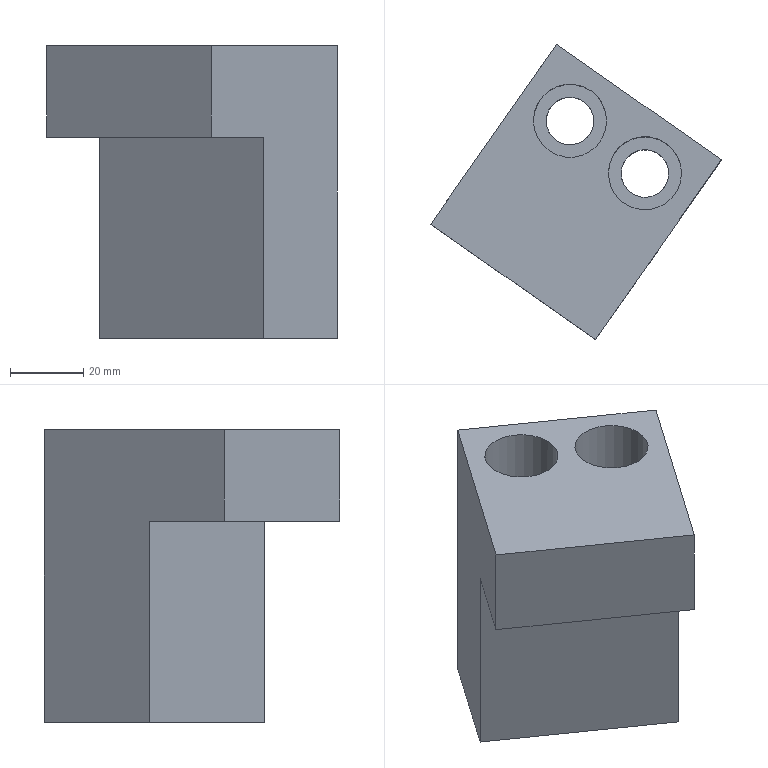Part | NX | features solid 2 | 1 solid | 14 faces | box 79.468 x 80.696 x 80 mm | volume 148999 mm3 | plane 9 | cylinder 4 | spline 1 | commonest cylinder face diameters 13 x2 20 x2
STEP:
#1=CARTESIAN_POINT('',(301.621,356.463,-125.));
#2=VERTEX_POINT('',#1);
#3=CARTESIAN_POINT('',(256.568,388.01,-125.));
#4=VERTEX_POINT('',#3);
#5=CARTESIAN_POINT('',(791.825,13.218,-125.));
#6=DIRECTION('',(-0.8192,0.5736,0.));
#7=VECTOR('',#6,1000.);
#8=LINE('',#5,#7);
#9=EDGE_CURVE('',#2,#4,#8,.T.);
#10=ORIENTED_EDGE('',*,*,#9,.F.);
#11=CARTESIAN_POINT('',(287.282,335.984,-125.));
#12=VERTEX_POINT('',#11);
#13=CARTESIAN_POINT('',(281.546,327.793,-125.));
#14=DIRECTION('',(-0.5736,-0.8192,0.));
#15=VECTOR('',#14,1000.);
#16=LINE('',#13,#15);
#17=EDGE_CURVE('',#12,#2,#16,.F.);
#18=ORIENTED_EDGE('',*,*,#17,.F.);
#19=CARTESIAN_POINT('',(242.228,367.531,-125.));
#20=VERTEX_POINT('',#19);
#21=CARTESIAN_POINT('',(283.186,338.852,-125.));
#22=DIRECTION('',(0.8192,-0.5736,0.));
#23=VECTOR('',#22,1000.);
#24=LINE('',#21,#23);
#25=EDGE_CURVE('',#12,#20,#24,.F.);
#26=ORIENTED_EDGE('',*,*,#25,.T.);
#27=CARTESIAN_POINT('',(-24.693,-13.672,-125.));
#28=DIRECTION('',(-0.5736,-0.8192,0.));
#29=VECTOR('',#28,1000.);
#30=LINE('',#27,#29);
#31=EDGE_CURVE('',#20,#4,#30,.F.);
#32=ORIENTED_EDGE('',*,*,#31,.T.);
#33=EDGE_LOOP('',(#10,#18,#26,#32));
#34=FACE_BOUND('',#33,.T.);
#35=CARTESIAN_POINT('',(510.565,-388.463,-125.));
#36=DIRECTION('',(0.,0.,-1.));
#37=DIRECTION('',(-0.342,0.9397,0.));
#38=AXIS2_PLACEMENT_3D('',#35,#36,#37);
#39=PLANE('',#38);
#40=ADVANCED_FACE('',(#34),#39,.T.);
#41=ORIENTED_EDGE('',*,*,#25,.F.);
#42=CARTESIAN_POINT('',(287.282,335.984,-100.));
#43=VERTEX_POINT('',#42);
#44=CARTESIAN_POINT('',(287.282,335.984,-100.));
#45=DIRECTION('',(0.,0.,-1.));
#46=VECTOR('',#45,1000.);
#47=LINE('',#44,#46);
#48=EDGE_CURVE('',#43,#12,#47,.T.);
#49=ORIENTED_EDGE('',*,*,#48,.F.);
#50=CARTESIAN_POINT('',(242.228,367.531,-100.));
#51=VERTEX_POINT('',#50);
#52=CARTESIAN_POINT('',(283.186,338.852,-100.));
#53=DIRECTION('',(0.8192,-0.5736,0.));
#54=VECTOR('',#53,1000.);
#55=LINE('',#52,#54);
#56=EDGE_CURVE('',#43,#51,#55,.F.);
#57=ORIENTED_EDGE('',*,*,#56,.T.);
#58=CARTESIAN_POINT('',(242.228,367.531,-100.));
#59=DIRECTION('',(0.,0.,-1.));
#60=VECTOR('',#59,1000.);
#61=LINE('',#58,#60);
#62=EDGE_CURVE('',#51,#20,#61,.T.);
#63=ORIENTED_EDGE('',*,*,#62,.T.);
#64=EDGE_LOOP('',(#41,#49,#57,#63));
#65=FACE_BOUND('',#64,.T.);
#66=CARTESIAN_POINT('',(283.186,338.852,-100.));
#67=DIRECTION('',(0.5736,0.8192,0.));
#68=DIRECTION('',(0.8192,-0.5736,0.));
#69=AXIS2_PLACEMENT_3D('',#66,#67,#68);
#70=PLANE('',#69);
#71=ADVANCED_FACE('',(#65),#70,.F.);
#72=ORIENTED_EDGE('',*,*,#31,.F.);
#73=ORIENTED_EDGE('',*,*,#62,.F.);
#74=CARTESIAN_POINT('',(276.643,416.68,-100.));
#75=VERTEX_POINT('',#74);
#76=CARTESIAN_POINT('',(-24.693,-13.672,-100.));
#77=DIRECTION('',(-0.5736,-0.8192,0.));
#78=VECTOR('',#77,1000.);
#79=LINE('',#76,#78);
#80=EDGE_CURVE('',#51,#75,#79,.F.);
#81=ORIENTED_EDGE('',*,*,#80,.T.);
#82=CARTESIAN_POINT('',(276.643,416.68,-180.));
#83=VERTEX_POINT('',#82);
#84=CARTESIAN_POINT('',(276.643,416.68,-100.));
#85=DIRECTION('',(0.,0.,-1.));
#86=VECTOR('',#85,1000.);
#87=LINE('',#84,#86);
#88=EDGE_CURVE('',#75,#83,#87,.T.);
#89=ORIENTED_EDGE('',*,*,#88,.T.);
#90=CARTESIAN_POINT('',(256.568,388.01,-180.));
#91=VERTEX_POINT('',#90);
#92=CARTESIAN_POINT('',(256.568,388.01,-180.));
#93=CARTESIAN_POINT('',(263.259,397.566,-180.));
#94=CARTESIAN_POINT('',(269.951,407.123,-180.));
#95=CARTESIAN_POINT('',(276.643,416.68,-180.));
#96=B_SPLINE_CURVE_WITH_KNOTS('',3,(#92,#93,#94,#95),.UNSPECIFIED.,.F.,.F.,(4,4),(0.,0.035),.UNSPECIFIED.);
#97=EDGE_CURVE('',#91,#83,#96,.T.);
#98=ORIENTED_EDGE('',*,*,#97,.F.);
#99=CARTESIAN_POINT('',(256.568,388.01,-175.));
#100=DIRECTION('',(0.,0.,-1.));
#101=VECTOR('',#100,1000.);
#102=LINE('',#99,#101);
#103=EDGE_CURVE('',#91,#4,#102,.F.);
#104=ORIENTED_EDGE('',*,*,#103,.T.);
#105=EDGE_LOOP('',(#72,#73,#81,#89,#98,#104));
#106=FACE_BOUND('',#105,.T.);
#107=CARTESIAN_POINT('',(-24.693,-13.672,-100.));
#108=DIRECTION('',(0.8192,-0.5736,0.));
#109=DIRECTION('',(-0.5736,-0.8192,0.));
#110=AXIS2_PLACEMENT_3D('',#107,#108,#109);
#111=PLANE('',#110);
#112=ADVANCED_FACE('',(#106),#111,.F.);
#113=CARTESIAN_POINT('',(321.696,385.133,-100.));
#114=VERTEX_POINT('',#113);
#115=CARTESIAN_POINT('',(321.696,385.133,-180.));
#116=VERTEX_POINT('',#115);
#117=CARTESIAN_POINT('',(321.696,385.133,-100.));
#118=DIRECTION('',(0.,0.,-1.));
#119=VECTOR('',#118,1000.);
#120=LINE('',#117,#119);
#121=EDGE_CURVE('',#114,#116,#120,.T.);
#122=ORIENTED_EDGE('',*,*,#121,.T.);
#123=CARTESIAN_POINT('',(321.696,385.133,-180.));
#124=CARTESIAN_POINT('',(306.678,395.649,-180.));
#125=CARTESIAN_POINT('',(291.661,406.164,-180.));
#126=CARTESIAN_POINT('',(276.643,416.68,-180.));
#127=B_SPLINE_CURVE_WITH_KNOTS('',3,(#123,#124,#125,#126),.UNSPECIFIED.,.F.,.F.,(4,4),(0.,0.055),.UNSPECIFIED.);
#128=EDGE_CURVE('',#116,#83,#127,.T.);
#129=ORIENTED_EDGE('',*,*,#128,.T.);
#130=ORIENTED_EDGE('',*,*,#88,.F.);
#131=CARTESIAN_POINT('',(313.505,390.869,-100.));
#132=DIRECTION('',(0.8192,-0.5736,0.));
#133=VECTOR('',#132,1000.);
#134=LINE('',#131,#133);
#135=EDGE_CURVE('',#114,#75,#134,.F.);
#136=ORIENTED_EDGE('',*,*,#135,.F.);
#137=EDGE_LOOP('',(#122,#129,#130,#136));
#138=FACE_BOUND('',#137,.T.);
#139=CARTESIAN_POINT('',(313.505,390.869,-15.));
#140=DIRECTION('',(0.5736,0.8192,0.));
#141=DIRECTION('',(0.8192,-0.5736,0.));
#142=AXIS2_PLACEMENT_3D('',#139,#140,#141);
#143=PLANE('',#142);
#144=ADVANCED_FACE('',(#138),#143,.T.);
#145=ORIENTED_EDGE('',*,*,#17,.T.);
#146=CARTESIAN_POINT('',(301.621,356.463,-180.));
#147=VERTEX_POINT('',#146);
#148=CARTESIAN_POINT('',(301.621,356.463,-175.));
#149=DIRECTION('',(0.,0.,-1.));
#150=VECTOR('',#149,1000.);
#151=LINE('',#148,#150);
#152=EDGE_CURVE('',#147,#2,#151,.F.);
#153=ORIENTED_EDGE('',*,*,#152,.F.);
#154=CARTESIAN_POINT('',(301.621,356.463,-180.));
#155=CARTESIAN_POINT('',(308.313,366.02,-180.));
#156=CARTESIAN_POINT('',(315.005,375.576,-180.));
#157=CARTESIAN_POINT('',(321.696,385.133,-180.));
#158=B_SPLINE_CURVE_WITH_KNOTS('',3,(#154,#155,#156,#157),.UNSPECIFIED.,.F.,.F.,(4,4),(0.,0.035),.UNSPECIFIED.);
#159=EDGE_CURVE('',#147,#116,#158,.T.);
#160=ORIENTED_EDGE('',*,*,#159,.T.);
#161=ORIENTED_EDGE('',*,*,#121,.F.);
#162=CARTESIAN_POINT('',(281.546,327.793,-100.));
#163=DIRECTION('',(-0.5736,-0.8192,0.));
#164=VECTOR('',#163,1000.);
#165=LINE('',#162,#164);
#166=EDGE_CURVE('',#43,#114,#165,.F.);
#167=ORIENTED_EDGE('',*,*,#166,.F.);
#168=ORIENTED_EDGE('',*,*,#48,.T.);
#169=EDGE_LOOP('',(#145,#153,#160,#161,#167,#168));
#170=FACE_BOUND('',#169,.T.);
#171=CARTESIAN_POINT('',(281.546,327.793,-100.));
#172=DIRECTION('',(0.8192,-0.5736,0.));
#173=DIRECTION('',(-0.5736,-0.8192,0.));
#174=AXIS2_PLACEMENT_3D('',#171,#172,#173);
#175=PLANE('',#174);
#176=ADVANCED_FACE('',(#170),#175,.T.);
#177=CARTESIAN_POINT('',(297.385,390.846,-100.));
#178=VERTEX_POINT('',#177);
#179=CARTESIAN_POINT('',(300.805,381.45,-100.));
#180=DIRECTION('',(0.,0.,1.));
#181=DIRECTION('',(-0.342,0.9397,0.));
#182=AXIS2_PLACEMENT_3D('',#179,#180,#181);
#183=CIRCLE('',#182,10.);
#184=EDGE_CURVE('',#178,#178,#183,.F.);
#185=ORIENTED_EDGE('',*,*,#184,.T.);
#186=EDGE_LOOP('',(#185));
#187=FACE_BOUND('',#186,.T.);
#188=CARTESIAN_POINT('',(276.906,405.186,-100.));
#189=VERTEX_POINT('',#188);
#190=CARTESIAN_POINT('',(280.326,395.789,-100.));
#191=DIRECTION('',(0.,0.,1.));
#192=DIRECTION('',(-0.342,0.9397,0.));
#193=AXIS2_PLACEMENT_3D('',#190,#191,#192);
#194=CIRCLE('',#193,10.);
#195=EDGE_CURVE('',#189,#189,#194,.F.);
#196=ORIENTED_EDGE('',*,*,#195,.T.);
#197=EDGE_LOOP('',(#196));
#198=FACE_BOUND('',#197,.T.);
#199=ORIENTED_EDGE('',*,*,#56,.F.);
#200=ORIENTED_EDGE('',*,*,#166,.T.);
#201=ORIENTED_EDGE('',*,*,#135,.T.);
#202=ORIENTED_EDGE('',*,*,#80,.F.);
#203=EDGE_LOOP('',(#199,#200,#201,#202));
#204=FACE_BOUND('',#203,.T.);
#205=CARTESIAN_POINT('',(510.565,-388.463,-100.));
#206=DIRECTION('',(0.,0.,-1.));
#207=DIRECTION('',(-0.342,0.9397,0.));
#208=AXIS2_PLACEMENT_3D('',#205,#206,#207);
#209=PLANE('',#208);
#210=ADVANCED_FACE('',(#187,#198,#204),#209,.F.);
#211=CARTESIAN_POINT('',(273.826,395.789,-150.));
#212=VERTEX_POINT('',#211);
#213=CARTESIAN_POINT('',(280.326,395.789,-150.));
#214=DIRECTION('',(0.,0.,-1.));
#215=DIRECTION('',(-1.,0.,0.));
#216=AXIS2_PLACEMENT_3D('',#213,#214,#215);
#217=CIRCLE('',#216,6.5);
#218=EDGE_CURVE('',#212,#212,#217,.T.);
#219=ORIENTED_EDGE('',*,*,#218,.F.);
#220=EDGE_LOOP('',(#219));
#221=FACE_BOUND('',#220,.T.);
#222=CARTESIAN_POINT('',(282.55,389.681,-180.));
#223=VERTEX_POINT('',#222);
#224=CARTESIAN_POINT('',(286.859,392.75,-180.));
#225=CARTESIAN_POINT('',(282.789,389.018,-180.));
#226=CARTESIAN_POINT('',(277.281,389.263,-180.));
#227=CARTESIAN_POINT('',(273.56,393.321,-180.));
#228=CARTESIAN_POINT('',(273.795,398.83,-180.));
#229=CARTESIAN_POINT('',(277.862,402.557,-180.));
#230=CARTESIAN_POINT('',(283.363,402.32,-180.));
#231=CARTESIAN_POINT('',(287.093,398.26,-180.));
#232=CARTESIAN_POINT('',(286.859,392.75,-180.));
#233=CARTESIAN_POINT('',(282.789,389.018,-180.));
#234=CARTESIAN_POINT('',(277.281,389.263,-180.));
#235=B_SPLINE_CURVE_WITH_KNOTS('',3,(#224,#225,#226,#227,#228,#229,#230,#231,#232,#233,#234),.UNSPECIFIED.,.T.,.F.,(1,1,1,1,1,1,1,1,1,1,1,1,1,1,1),(-0.01524,-0.01016,-0.00508,0.,0.00508,0.01016,0.01524,0.02032,0.0254,0.03048,0.03556,0.04064,0.04572,0.0508,0.05588),.UNSPECIFIED.);
#236=EDGE_CURVE('',#223,#223,#235,.T.);
#237=ORIENTED_EDGE('',*,*,#236,.T.);
#238=EDGE_LOOP('',(#237));
#239=FACE_BOUND('',#238,.T.);
#240=CARTESIAN_POINT('',(280.326,395.789,-145.));
#241=DIRECTION('',(0.,0.,1.));
#242=DIRECTION('',(0.342,-0.9397,0.));
#243=AXIS2_PLACEMENT_3D('',#240,#241,#242);
#244=CYLINDRICAL_SURFACE('',#243,6.5);
#245=ADVANCED_FACE('',(#221,#239),#244,.F.);
#246=ORIENTED_EDGE('',*,*,#218,.T.);
#247=EDGE_LOOP('',(#246));
#248=FACE_BOUND('',#247,.T.);
#249=CARTESIAN_POINT('',(270.326,395.789,-150.));
#250=VERTEX_POINT('',#249);
#251=CARTESIAN_POINT('',(280.326,395.789,-150.));
#252=DIRECTION('',(0.,0.,-1.));
#253=DIRECTION('',(-1.,0.,0.));
#254=AXIS2_PLACEMENT_3D('',#251,#252,#253);
#255=CIRCLE('',#254,10.);
#256=EDGE_CURVE('',#250,#250,#255,.T.);
#257=ORIENTED_EDGE('',*,*,#256,.F.);
#258=EDGE_LOOP('',(#257));
#259=FACE_BOUND('',#258,.T.);
#260=CARTESIAN_POINT('',(280.326,395.789,-150.));
#261=DIRECTION('',(0.,0.,-1.));
#262=DIRECTION('',(-0.342,0.9397,0.));
#263=AXIS2_PLACEMENT_3D('',#260,#261,#262);
#264=PLANE('',#263);
#265=ADVANCED_FACE('',(#248,#259),#264,.F.);
#266=ORIENTED_EDGE('',*,*,#195,.F.);
#267=EDGE_LOOP('',(#266));
#268=FACE_BOUND('',#267,.T.);
#269=ORIENTED_EDGE('',*,*,#256,.T.);
#270=EDGE_LOOP('',(#269));
#271=FACE_BOUND('',#270,.T.);
#272=CARTESIAN_POINT('',(280.326,395.789,-105.));
#273=DIRECTION('',(0.,0.,1.));
#274=DIRECTION('',(0.342,-0.9397,0.));
#275=AXIS2_PLACEMENT_3D('',#272,#273,#274);
#276=CYLINDRICAL_SURFACE('',#275,10.);
#277=ADVANCED_FACE('',(#268,#271),#276,.F.);
#278=CARTESIAN_POINT('',(294.305,381.45,-150.));
#279=VERTEX_POINT('',#278);
#280=CARTESIAN_POINT('',(300.805,381.45,-150.));
#281=DIRECTION('',(0.,0.,-1.));
#282=DIRECTION('',(-1.,0.,0.));
#283=AXIS2_PLACEMENT_3D('',#280,#281,#282);
#284=CIRCLE('',#283,6.5);
#285=EDGE_CURVE('',#279,#279,#284,.T.);
#286=ORIENTED_EDGE('',*,*,#285,.F.);
#287=EDGE_LOOP('',(#286));
#288=FACE_BOUND('',#287,.T.);
#289=CARTESIAN_POINT('',(303.028,375.342,-180.));
#290=VERTEX_POINT('',#289);
#291=CARTESIAN_POINT('',(307.338,378.411,-180.));
#292=CARTESIAN_POINT('',(303.268,374.679,-180.));
#293=CARTESIAN_POINT('',(297.76,374.923,-180.));
#294=CARTESIAN_POINT('',(294.039,378.981,-180.));
#295=CARTESIAN_POINT('',(294.274,384.491,-180.));
#296=CARTESIAN_POINT('',(298.341,388.217,-180.));
#297=CARTESIAN_POINT('',(303.842,387.98,-180.));
#298=CARTESIAN_POINT('',(307.572,383.921,-180.));
#299=CARTESIAN_POINT('',(307.338,378.411,-180.));
#300=CARTESIAN_POINT('',(303.268,374.679,-180.));
#301=CARTESIAN_POINT('',(297.76,374.923,-180.));
#302=B_SPLINE_CURVE_WITH_KNOTS('',3,(#291,#292,#293,#294,#295,#296,#297,#298,#299,#300,#301),.UNSPECIFIED.,.T.,.F.,(1,1,1,1,1,1,1,1,1,1,1,1,1,1,1),(-0.01524,-0.01016,-0.00508,0.,0.00508,0.01016,0.01524,0.02032,0.0254,0.03048,0.03556,0.04064,0.04572,0.0508,0.05588),.UNSPECIFIED.);
#303=EDGE_CURVE('',#290,#290,#302,.T.);
#304=ORIENTED_EDGE('',*,*,#303,.T.);
#305=EDGE_LOOP('',(#304));
#306=FACE_BOUND('',#305,.T.);
#307=CARTESIAN_POINT('',(300.805,381.45,-145.));
#308=DIRECTION('',(0.,0.,1.));
#309=DIRECTION('',(0.342,-0.9397,0.));
#310=AXIS2_PLACEMENT_3D('',#307,#308,#309);
#311=CYLINDRICAL_SURFACE('',#310,6.5);
#312=ADVANCED_FACE('',(#288,#306),#311,.F.);
#313=ORIENTED_EDGE('',*,*,#285,.T.);
#314=EDGE_LOOP('',(#313));
#315=FACE_BOUND('',#314,.T.);
#316=CARTESIAN_POINT('',(290.805,381.45,-150.));
#317=VERTEX_POINT('',#316);
#318=CARTESIAN_POINT('',(300.805,381.45,-150.));
#319=DIRECTION('',(0.,0.,-1.));
#320=DIRECTION('',(-1.,0.,0.));
#321=AXIS2_PLACEMENT_3D('',#318,#319,#320);
#322=CIRCLE('',#321,10.);
#323=EDGE_CURVE('',#317,#317,#322,.T.);
#324=ORIENTED_EDGE('',*,*,#323,.F.);
#325=EDGE_LOOP('',(#324));
#326=FACE_BOUND('',#325,.T.);
#327=CARTESIAN_POINT('',(300.805,381.45,-150.));
#328=DIRECTION('',(0.,0.,-1.));
#329=DIRECTION('',(-0.342,0.9397,0.));
#330=AXIS2_PLACEMENT_3D('',#327,#328,#329);
#331=PLANE('',#330);
#332=ADVANCED_FACE('',(#315,#326),#331,.F.);
#333=ORIENTED_EDGE('',*,*,#184,.F.);
#334=EDGE_LOOP('',(#333));
#335=FACE_BOUND('',#334,.T.);
#336=ORIENTED_EDGE('',*,*,#323,.T.);
#337=EDGE_LOOP('',(#336));
#338=FACE_BOUND('',#337,.T.);
#339=CARTESIAN_POINT('',(300.805,381.45,-105.));
#340=DIRECTION('',(0.,0.,1.));
#341=DIRECTION('',(0.342,-0.9397,0.));
#342=AXIS2_PLACEMENT_3D('',#339,#340,#341);
#343=CYLINDRICAL_SURFACE('',#342,10.);
#344=ADVANCED_FACE('',(#335,#338),#343,.F.);
#345=ORIENTED_EDGE('',*,*,#9,.T.);
#346=ORIENTED_EDGE('',*,*,#103,.F.);
#347=CARTESIAN_POINT('',(301.621,356.463,-180.));
#348=CARTESIAN_POINT('',(286.603,366.978,-180.));
#349=CARTESIAN_POINT('',(271.585,377.494,-180.));
#350=CARTESIAN_POINT('',(256.568,388.01,-180.));
#351=B_SPLINE_CURVE_WITH_KNOTS('',3,(#347,#348,#349,#350),.UNSPECIFIED.,.F.,.F.,(4,4),(0.,0.055),.UNSPECIFIED.);
#352=EDGE_CURVE('',#147,#91,#351,.T.);
#353=ORIENTED_EDGE('',*,*,#352,.F.);
#354=ORIENTED_EDGE('',*,*,#152,.T.);
#355=EDGE_LOOP('',(#345,#346,#353,#354));
#356=FACE_BOUND('',#355,.T.);
#357=CARTESIAN_POINT('',(289.334,365.066,-15.));
#358=DIRECTION('',(-0.5736,-0.8192,0.));
#359=DIRECTION('',(0.8192,-0.5736,0.));
#360=AXIS2_PLACEMENT_3D('',#357,#358,#359);
#361=PLANE('',#360);
#362=ADVANCED_FACE('',(#356),#361,.T.);
#363=ORIENTED_EDGE('',*,*,#303,.F.);
#364=EDGE_LOOP('',(#363));
#365=FACE_BOUND('',#364,.T.);
#366=ORIENTED_EDGE('',*,*,#236,.F.);
#367=EDGE_LOOP('',(#366));
#368=FACE_BOUND('',#367,.T.);
#369=ORIENTED_EDGE('',*,*,#352,.T.);
#370=ORIENTED_EDGE('',*,*,#97,.T.);
#371=ORIENTED_EDGE('',*,*,#128,.F.);
#372=ORIENTED_EDGE('',*,*,#159,.F.);
#373=EDGE_LOOP('',(#369,#370,#371,#372));
#374=FACE_BOUND('',#373,.T.);
#375=CARTESIAN_POINT('',(322.087,356.102,-180.));
#376=CARTESIAN_POINT('',(256.177,356.102,-180.));
#377=CARTESIAN_POINT('',(322.087,357.401,-180.));
#378=CARTESIAN_POINT('',(256.177,357.401,-180.));
#379=CARTESIAN_POINT('',(322.087,358.701,-180.));
#380=CARTESIAN_POINT('',(256.177,358.701,-180.));
#381=CARTESIAN_POINT('',(322.087,360.,-180.));
#382=CARTESIAN_POINT('',(256.177,360.,-180.));
#383=CARTESIAN_POINT('',(322.087,379.014,-180.));
#384=CARTESIAN_POINT('',(256.177,379.014,-180.));
#385=CARTESIAN_POINT('',(322.087,398.027,-180.));
#386=CARTESIAN_POINT('',(256.177,398.027,-180.));
#387=CARTESIAN_POINT('',(322.087,417.041,-180.));
#388=CARTESIAN_POINT('',(256.177,417.041,-180.));
#389=B_SPLINE_SURFACE_WITH_KNOTS('',3,1,((#375,#376),(#377,#378),(#379,#380),(#381,#382),(#383,#384),(#385,#386),(#387,#388)),.SURF_OF_LINEAR_EXTRUSION.,.F.,.F.,.F.,(4,3,4),(2,2),(-0.008475,0.,0.124),(0.,1.),.PIECEWISE_BEZIER_KNOTS.);
#390=ADVANCED_FACE('',(#365,#368,#374),#389,.F.);
#391=CLOSED_SHELL('',(#40,#71,#112,#144,#176,#210,#245,#265,#277,#312,#332,#344,#362,#390));
#392=MANIFOLD_SOLID_BREP('',#391);
#393=(LENGTH_UNIT()NAMED_UNIT(*)SI_UNIT(.MILLI.,.METRE.));
#394=UNCERTAINTY_MEASURE_WITH_UNIT(LENGTH_MEASURE(0.0508),#393,'','');
#395=(NAMED_UNIT(*)PLANE_ANGLE_UNIT()SI_UNIT($,.RADIAN.));
#396=(NAMED_UNIT(*)SI_UNIT($,.STERADIAN.)SOLID_ANGLE_UNIT());
#397=(GEOMETRIC_REPRESENTATION_CONTEXT(3)GLOBAL_UNCERTAINTY_ASSIGNED_CONTEXT((#394))GLOBAL_UNIT_ASSIGNED_CONTEXT((#393,#395,#396))REPRESENTATION_CONTEXT('',''));
#398=ADVANCED_BREP_SHAPE_REPRESENTATION('',(#392),#397);